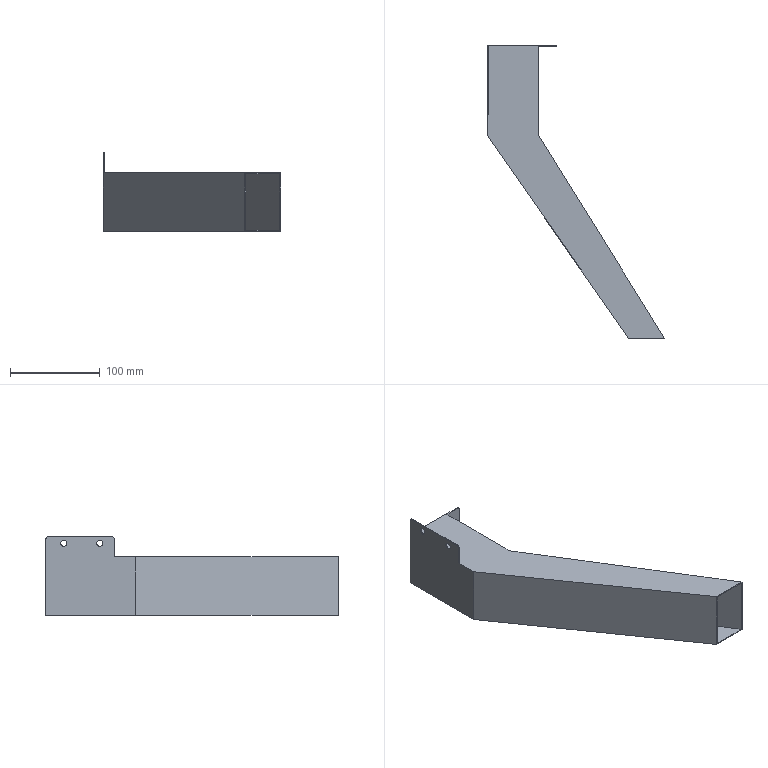Part | NX | 1 solid | 35 faces | box 197 x 325 x 87.5 mm | volume 82670 mm3 | plane 19 | cylinder 12 | cone 4 | commonest cylinder face diameters 6 x4 6.4 x4 7 x4
STEP:
#1=CARTESIAN_POINT('',(1114.,-232.5,-79.28));
#2=VERTEX_POINT('',#1);
#3=CARTESIAN_POINT('',(1271.,-457.5,-79.28));
#4=VERTEX_POINT('',#3);
#5=CARTESIAN_POINT('',(1002.386,-72.544,-79.28));
#6=DIRECTION('',(0.5722,-0.8201,0.));
#7=VECTOR('',#6,1000.);
#8=LINE('',#5,#7);
#9=EDGE_CURVE('',#2,#4,#8,.T.);
#10=ORIENTED_EDGE('',*,*,#9,.F.);
#11=CARTESIAN_POINT('',(1114.,-232.5,-144.28));
#12=VERTEX_POINT('',#11);
#13=CARTESIAN_POINT('',(1114.,-232.5,-79.28));
#14=DIRECTION('',(0.,0.,-1.));
#15=VECTOR('',#14,1000.);
#16=LINE('',#13,#15);
#17=EDGE_CURVE('',#2,#12,#16,.T.);
#18=ORIENTED_EDGE('',*,*,#17,.T.);
#19=CARTESIAN_POINT('',(1271.,-457.5,-144.28));
#20=VERTEX_POINT('',#19);
#21=CARTESIAN_POINT('',(1002.386,-72.544,-144.28));
#22=DIRECTION('',(0.5722,-0.8201,0.));
#23=VECTOR('',#22,1000.);
#24=LINE('',#21,#23);
#25=EDGE_CURVE('',#12,#20,#24,.T.);
#26=ORIENTED_EDGE('',*,*,#25,.T.);
#27=CARTESIAN_POINT('',(1271.,-457.5,-79.28));
#28=DIRECTION('',(0.,0.,1.));
#29=VECTOR('',#28,1000.);
#30=LINE('',#27,#29);
#31=EDGE_CURVE('',#20,#4,#30,.T.);
#32=ORIENTED_EDGE('',*,*,#31,.T.);
#33=EDGE_LOOP('',(#10,#18,#26,#32));
#34=FACE_BOUND('',#33,.T.);
#35=CARTESIAN_POINT('',(1114.,-232.5,-79.28));
#36=DIRECTION('',(-0.8201,-0.5722,0.));
#37=DIRECTION('',(-0.5722,0.8201,0.));
#38=AXIS2_PLACEMENT_3D('',#35,#36,#37);
#39=PLANE('',#38);
#40=ADVANCED_FACE('',(#34),#39,.T.);
#41=CARTESIAN_POINT('',(1114.,-132.5,-144.28));
#42=VERTEX_POINT('',#41);
#43=CARTESIAN_POINT('',(1114.,-132.5,-59.78));
#44=VERTEX_POINT('',#43);
#45=CARTESIAN_POINT('',(1114.,-132.5,-79.28));
#46=DIRECTION('',(0.,0.,1.));
#47=VECTOR('',#46,1000.);
#48=LINE('',#45,#47);
#49=EDGE_CURVE('',#42,#44,#48,.T.);
#50=ORIENTED_EDGE('',*,*,#49,.F.);
#51=CARTESIAN_POINT('',(1114.,-232.5,-144.28));
#52=DIRECTION('',(0.,1.,0.));
#53=VECTOR('',#52,1000.);
#54=LINE('',#51,#53);
#55=EDGE_CURVE('',#12,#42,#54,.T.);
#56=ORIENTED_EDGE('',*,*,#55,.F.);
#57=ORIENTED_EDGE('',*,*,#17,.F.);
#58=CARTESIAN_POINT('',(1114.,-208.721,-79.28));
#59=VERTEX_POINT('',#58);
#60=CARTESIAN_POINT('',(1114.,-232.5,-79.28));
#61=DIRECTION('',(0.,1.,0.));
#62=VECTOR('',#61,1000.);
#63=LINE('',#60,#62);
#64=EDGE_CURVE('',#2,#59,#63,.T.);
#65=ORIENTED_EDGE('',*,*,#64,.T.);
#66=CARTESIAN_POINT('',(1114.,-208.721,-59.78));
#67=VERTEX_POINT('',#66);
#68=CARTESIAN_POINT('',(1114.,-208.721,-79.28));
#69=DIRECTION('',(0.,0.,1.));
#70=VECTOR('',#69,1000.);
#71=LINE('',#68,#70);
#72=EDGE_CURVE('',#59,#67,#71,.T.);
#73=ORIENTED_EDGE('',*,*,#72,.T.);
#74=CARTESIAN_POINT('',(1114.,-205.721,-56.78));
#75=VERTEX_POINT('',#74);
#76=CARTESIAN_POINT('',(1114.,-205.721,-59.78));
#77=DIRECTION('',(-1.,0.,0.));
#78=DIRECTION('',(0.,1.,0.));
#79=AXIS2_PLACEMENT_3D('',#76,#77,#78);
#80=CIRCLE('',#79,3.);
#81=EDGE_CURVE('',#67,#75,#80,.T.);
#82=ORIENTED_EDGE('',*,*,#81,.T.);
#83=CARTESIAN_POINT('',(1114.,-135.5,-56.78));
#84=VERTEX_POINT('',#83);
#85=CARTESIAN_POINT('',(1114.,-72.544,-56.78));
#86=DIRECTION('',(0.,1.,0.));
#87=VECTOR('',#86,1000.);
#88=LINE('',#85,#87);
#89=EDGE_CURVE('',#75,#84,#88,.T.);
#90=ORIENTED_EDGE('',*,*,#89,.T.);
#91=CARTESIAN_POINT('',(1114.,-135.5,-59.78));
#92=DIRECTION('',(1.,0.,0.));
#93=DIRECTION('',(0.,-1.,0.));
#94=AXIS2_PLACEMENT_3D('',#91,#92,#93);
#95=CIRCLE('',#94,3.);
#96=EDGE_CURVE('',#44,#84,#95,.T.);
#97=ORIENTED_EDGE('',*,*,#96,.F.);
#98=EDGE_LOOP('',(#50,#56,#57,#65,#73,#82,#90,#97));
#99=FACE_BOUND('',#98,.T.);
#100=CARTESIAN_POINT('',(1114.,-149.,-64.28));
#101=VERTEX_POINT('',#100);
#102=CARTESIAN_POINT('',(1114.,-156.,-64.28));
#103=VERTEX_POINT('',#102);
#104=CARTESIAN_POINT('',(1114.,-152.5,-64.28));
#105=DIRECTION('',(1.,0.,0.));
#106=DIRECTION('',(0.,-1.,0.));
#107=AXIS2_PLACEMENT_3D('',#104,#105,#106);
#108=CIRCLE('',#107,3.5);
#109=EDGE_CURVE('',#101,#103,#108,.T.);
#110=ORIENTED_EDGE('',*,*,#109,.T.);
#111=CARTESIAN_POINT('',(1114.,-152.5,-64.28));
#112=DIRECTION('',(1.,0.,0.));
#113=DIRECTION('',(0.,-1.,0.));
#114=AXIS2_PLACEMENT_3D('',#111,#112,#113);
#115=CIRCLE('',#114,3.5);
#116=EDGE_CURVE('',#103,#101,#115,.T.);
#117=ORIENTED_EDGE('',*,*,#116,.T.);
#118=EDGE_LOOP('',(#110,#117));
#119=FACE_BOUND('',#118,.T.);
#120=CARTESIAN_POINT('',(1114.,-189.,-64.28));
#121=VERTEX_POINT('',#120);
#122=CARTESIAN_POINT('',(1114.,-196.,-64.28));
#123=VERTEX_POINT('',#122);
#124=CARTESIAN_POINT('',(1114.,-192.5,-64.28));
#125=DIRECTION('',(1.,0.,0.));
#126=DIRECTION('',(0.,-1.,0.));
#127=AXIS2_PLACEMENT_3D('',#124,#125,#126);
#128=CIRCLE('',#127,3.5);
#129=EDGE_CURVE('',#121,#123,#128,.T.);
#130=ORIENTED_EDGE('',*,*,#129,.T.);
#131=CARTESIAN_POINT('',(1114.,-192.5,-64.28));
#132=DIRECTION('',(1.,0.,0.));
#133=DIRECTION('',(0.,-1.,0.));
#134=AXIS2_PLACEMENT_3D('',#131,#132,#133);
#135=CIRCLE('',#134,3.5);
#136=EDGE_CURVE('',#123,#121,#135,.T.);
#137=ORIENTED_EDGE('',*,*,#136,.T.);
#138=EDGE_LOOP('',(#130,#137));
#139=FACE_BOUND('',#138,.T.);
#140=CARTESIAN_POINT('',(1114.,-132.5,-79.28));
#141=DIRECTION('',(-1.,0.,0.));
#142=DIRECTION('',(0.,0.,1.));
#143=AXIS2_PLACEMENT_3D('',#140,#141,#142);
#144=PLANE('',#143);
#145=ADVANCED_FACE('',(#99,#119,#139),#144,.T.);
#146=CARTESIAN_POINT('',(1191.,-132.5,-82.28));
#147=VERTEX_POINT('',#146);
#148=CARTESIAN_POINT('',(1191.,-132.5,-141.28));
#149=VERTEX_POINT('',#148);
#150=CARTESIAN_POINT('',(1191.,-132.5,-130.28));
#151=DIRECTION('',(0.,0.,-1.));
#152=VECTOR('',#151,1000.);
#153=LINE('',#150,#152);
#154=EDGE_CURVE('',#147,#149,#153,.T.);
#155=ORIENTED_EDGE('',*,*,#154,.F.);
#156=CARTESIAN_POINT('',(1191.,-133.5,-82.28));
#157=VERTEX_POINT('',#156);
#158=CARTESIAN_POINT('',(1191.,-132.5,-82.28));
#159=DIRECTION('',(0.,-1.,0.));
#160=VECTOR('',#159,1000.);
#161=LINE('',#158,#160);
#162=EDGE_CURVE('',#147,#157,#161,.T.);
#163=ORIENTED_EDGE('',*,*,#162,.T.);
#164=CARTESIAN_POINT('',(1191.,-133.5,-141.28));
#165=VERTEX_POINT('',#164);
#166=CARTESIAN_POINT('',(1191.,-133.5,-130.28));
#167=DIRECTION('',(0.,0.,-1.));
#168=VECTOR('',#167,1000.);
#169=LINE('',#166,#168);
#170=EDGE_CURVE('',#157,#165,#169,.T.);
#171=ORIENTED_EDGE('',*,*,#170,.T.);
#172=CARTESIAN_POINT('',(1191.,-132.5,-141.28));
#173=DIRECTION('',(0.,-1.,0.));
#174=VECTOR('',#173,1000.);
#175=LINE('',#172,#174);
#176=EDGE_CURVE('',#149,#165,#175,.T.);
#177=ORIENTED_EDGE('',*,*,#176,.F.);
#178=EDGE_LOOP('',(#155,#163,#171,#177));
#179=FACE_BOUND('',#178,.T.);
#180=CARTESIAN_POINT('',(1191.,-132.5,-82.28));
#181=DIRECTION('',(1.,0.,0.));
#182=DIRECTION('',(0.,1.,0.));
#183=AXIS2_PLACEMENT_3D('',#180,#181,#182);
#184=PLANE('',#183);
#185=ADVANCED_FACE('',(#179),#184,.T.);
#186=CARTESIAN_POINT('',(1171.,-133.5,-79.28));
#187=VERTEX_POINT('',#186);
#188=CARTESIAN_POINT('',(1171.,-232.5,-79.28));
#189=VERTEX_POINT('',#188);
#190=CARTESIAN_POINT('',(1171.,-132.5,-79.28));
#191=DIRECTION('',(0.,-1.,0.));
#192=VECTOR('',#191,1000.);
#193=LINE('',#190,#192);
#194=EDGE_CURVE('',#187,#189,#193,.T.);
#195=ORIENTED_EDGE('',*,*,#194,.T.);
#196=CARTESIAN_POINT('',(1171.,-232.5,-144.28));
#197=VERTEX_POINT('',#196);
#198=CARTESIAN_POINT('',(1171.,-232.5,-79.28));
#199=DIRECTION('',(0.,0.,-1.));
#200=VECTOR('',#199,1000.);
#201=LINE('',#198,#200);
#202=EDGE_CURVE('',#189,#197,#201,.T.);
#203=ORIENTED_EDGE('',*,*,#202,.T.);
#204=CARTESIAN_POINT('',(1171.,-133.5,-144.28));
#205=VERTEX_POINT('',#204);
#206=CARTESIAN_POINT('',(1171.,-132.5,-144.28));
#207=DIRECTION('',(0.,-1.,0.));
#208=VECTOR('',#207,1000.);
#209=LINE('',#206,#208);
#210=EDGE_CURVE('',#205,#197,#209,.T.);
#211=ORIENTED_EDGE('',*,*,#210,.F.);
#212=CARTESIAN_POINT('',(1171.,-133.5,-79.28));
#213=DIRECTION('',(0.,0.,1.));
#214=VECTOR('',#213,1000.);
#215=LINE('',#212,#214);
#216=EDGE_CURVE('',#205,#187,#215,.T.);
#217=ORIENTED_EDGE('',*,*,#216,.T.);
#218=EDGE_LOOP('',(#195,#203,#211,#217));
#219=FACE_BOUND('',#218,.T.);
#220=CARTESIAN_POINT('',(1171.,-232.5,-79.28));
#221=DIRECTION('',(1.,0.,0.));
#222=DIRECTION('',(0.,1.,0.));
#223=AXIS2_PLACEMENT_3D('',#220,#221,#222);
#224=PLANE('',#223);
#225=ADVANCED_FACE('',(#219),#224,.T.);
#226=CARTESIAN_POINT('',(1311.,-457.5,-79.28));
#227=VERTEX_POINT('',#226);
#228=CARTESIAN_POINT('',(1071.472,-72.544,-79.28));
#229=DIRECTION('',(0.5283,-0.8491,0.));
#230=VECTOR('',#229,1000.);
#231=LINE('',#228,#230);
#232=EDGE_CURVE('',#189,#227,#231,.T.);
#233=ORIENTED_EDGE('',*,*,#232,.T.);
#234=CARTESIAN_POINT('',(1311.,-457.5,-144.28));
#235=VERTEX_POINT('',#234);
#236=CARTESIAN_POINT('',(1311.,-457.5,-79.28));
#237=DIRECTION('',(0.,0.,-1.));
#238=VECTOR('',#237,1000.);
#239=LINE('',#236,#238);
#240=EDGE_CURVE('',#227,#235,#239,.T.);
#241=ORIENTED_EDGE('',*,*,#240,.T.);
#242=CARTESIAN_POINT('',(1071.472,-72.544,-144.28));
#243=DIRECTION('',(0.5283,-0.8491,0.));
#244=VECTOR('',#243,1000.);
#245=LINE('',#242,#244);
#246=EDGE_CURVE('',#197,#235,#245,.T.);
#247=ORIENTED_EDGE('',*,*,#246,.F.);
#248=ORIENTED_EDGE('',*,*,#202,.F.);
#249=EDGE_LOOP('',(#233,#241,#247,#248));
#250=FACE_BOUND('',#249,.T.);
#251=CARTESIAN_POINT('',(1311.,-457.5,-79.28));
#252=DIRECTION('',(0.8491,0.5283,0.));
#253=DIRECTION('',(0.,0.,-1.));
#254=AXIS2_PLACEMENT_3D('',#251,#252,#253);
#255=PLANE('',#254);
#256=ADVANCED_FACE('',(#250),#255,.T.);
#257=CARTESIAN_POINT('',(1140.033,-457.5,-79.28));
#258=DIRECTION('',(1.,0.,0.));
#259=VECTOR('',#258,1000.);
#260=LINE('',#257,#259);
#261=EDGE_CURVE('',#4,#227,#260,.T.);
#262=ORIENTED_EDGE('',*,*,#261,.F.);
#263=ORIENTED_EDGE('',*,*,#31,.F.);
#264=CARTESIAN_POINT('',(1140.033,-457.5,-144.28));
#265=DIRECTION('',(1.,0.,0.));
#266=VECTOR('',#265,1000.);
#267=LINE('',#264,#266);
#268=EDGE_CURVE('',#20,#235,#267,.T.);
#269=ORIENTED_EDGE('',*,*,#268,.T.);
#270=ORIENTED_EDGE('',*,*,#240,.F.);
#271=EDGE_LOOP('',(#262,#263,#269,#270));
#272=FACE_BOUND('',#271,.T.);
#273=CARTESIAN_POINT('',(1309.822,-457.5,-80.28));
#274=VERTEX_POINT('',#273);
#275=CARTESIAN_POINT('',(1309.822,-457.5,-143.28));
#276=VERTEX_POINT('',#275);
#277=CARTESIAN_POINT('',(1309.822,-457.5,-79.28));
#278=DIRECTION('',(0.,0.,-1.));
#279=VECTOR('',#278,1000.);
#280=LINE('',#277,#279);
#281=EDGE_CURVE('',#274,#276,#280,.T.);
#282=ORIENTED_EDGE('',*,*,#281,.T.);
#283=CARTESIAN_POINT('',(1272.219,-457.5,-143.28));
#284=VERTEX_POINT('',#283);
#285=CARTESIAN_POINT('',(1140.033,-457.5,-143.28));
#286=DIRECTION('',(1.,0.,0.));
#287=VECTOR('',#286,1000.);
#288=LINE('',#285,#287);
#289=EDGE_CURVE('',#284,#276,#288,.T.);
#290=ORIENTED_EDGE('',*,*,#289,.F.);
#291=CARTESIAN_POINT('',(1272.219,-457.5,-80.28));
#292=VERTEX_POINT('',#291);
#293=CARTESIAN_POINT('',(1272.219,-457.5,-79.28));
#294=DIRECTION('',(0.,0.,1.));
#295=VECTOR('',#294,1000.);
#296=LINE('',#293,#295);
#297=EDGE_CURVE('',#284,#292,#296,.T.);
#298=ORIENTED_EDGE('',*,*,#297,.T.);
#299=CARTESIAN_POINT('',(1140.033,-457.5,-80.28));
#300=DIRECTION('',(1.,0.,0.));
#301=VECTOR('',#300,1000.);
#302=LINE('',#299,#301);
#303=EDGE_CURVE('',#292,#274,#302,.T.);
#304=ORIENTED_EDGE('',*,*,#303,.T.);
#305=EDGE_LOOP('',(#282,#290,#298,#304));
#306=FACE_BOUND('',#305,.T.);
#307=CARTESIAN_POINT('',(1271.,-457.5,-79.28));
#308=DIRECTION('',(0.,-1.,0.));
#309=DIRECTION('',(0.,0.,-1.));
#310=AXIS2_PLACEMENT_3D('',#307,#308,#309);
#311=PLANE('',#310);
#312=ADVANCED_FACE('',(#272,#306),#311,.T.);
#313=ORIENTED_EDGE('',*,*,#303,.F.);
#314=CARTESIAN_POINT('',(1115.,-232.186,-80.28));
#315=VERTEX_POINT('',#314);
#316=CARTESIAN_POINT('',(1003.606,-72.544,-80.28));
#317=DIRECTION('',(-0.5722,0.8201,0.));
#318=VECTOR('',#317,1000.);
#319=LINE('',#316,#318);
#320=EDGE_CURVE('',#292,#315,#319,.T.);
#321=ORIENTED_EDGE('',*,*,#320,.T.);
#322=CARTESIAN_POINT('',(1115.,-132.5,-80.28));
#323=VERTEX_POINT('',#322);
#324=CARTESIAN_POINT('',(1115.,-72.544,-80.28));
#325=DIRECTION('',(0.,1.,0.));
#326=VECTOR('',#325,1000.);
#327=LINE('',#324,#326);
#328=EDGE_CURVE('',#315,#323,#327,.T.);
#329=ORIENTED_EDGE('',*,*,#328,.T.);
#330=CARTESIAN_POINT('',(1170.,-132.5,-80.28));
#331=VERTEX_POINT('',#330);
#332=CARTESIAN_POINT('',(1140.033,-132.5,-80.28));
#333=DIRECTION('',(1.,0.,0.));
#334=VECTOR('',#333,1000.);
#335=LINE('',#332,#334);
#336=EDGE_CURVE('',#323,#331,#335,.T.);
#337=ORIENTED_EDGE('',*,*,#336,.T.);
#338=CARTESIAN_POINT('',(1170.,-232.786,-80.28));
#339=VERTEX_POINT('',#338);
#340=CARTESIAN_POINT('',(1170.,-132.5,-80.28));
#341=DIRECTION('',(0.,-1.,0.));
#342=VECTOR('',#341,1000.);
#343=LINE('',#340,#342);
#344=EDGE_CURVE('',#331,#339,#343,.T.);
#345=ORIENTED_EDGE('',*,*,#344,.T.);
#346=CARTESIAN_POINT('',(1070.294,-72.544,-80.28));
#347=DIRECTION('',(0.5283,-0.8491,0.));
#348=VECTOR('',#347,1000.);
#349=LINE('',#346,#348);
#350=EDGE_CURVE('',#339,#274,#349,.T.);
#351=ORIENTED_EDGE('',*,*,#350,.T.);
#352=EDGE_LOOP('',(#313,#321,#329,#337,#345,#351));
#353=FACE_BOUND('',#352,.T.);
#354=CARTESIAN_POINT('',(1140.033,-72.544,-80.28));
#355=DIRECTION('',(0.,0.,1.));
#356=DIRECTION('',(1.,0.,0.));
#357=AXIS2_PLACEMENT_3D('',#354,#355,#356);
#358=PLANE('',#357);
#359=ADVANCED_FACE('',(#353),#358,.F.);
#360=CARTESIAN_POINT('',(1170.,-232.786,-143.28));
#361=VERTEX_POINT('',#360);
#362=CARTESIAN_POINT('',(1070.294,-72.544,-143.28));
#363=DIRECTION('',(0.5283,-0.8491,0.));
#364=VECTOR('',#363,1000.);
#365=LINE('',#362,#364);
#366=EDGE_CURVE('',#361,#276,#365,.T.);
#367=ORIENTED_EDGE('',*,*,#366,.F.);
#368=CARTESIAN_POINT('',(1170.,-132.5,-143.28));
#369=VERTEX_POINT('',#368);
#370=CARTESIAN_POINT('',(1170.,-72.544,-143.28));
#371=DIRECTION('',(0.,-1.,0.));
#372=VECTOR('',#371,1000.);
#373=LINE('',#370,#372);
#374=EDGE_CURVE('',#369,#361,#373,.T.);
#375=ORIENTED_EDGE('',*,*,#374,.F.);
#376=CARTESIAN_POINT('',(1115.,-132.5,-143.28));
#377=VERTEX_POINT('',#376);
#378=CARTESIAN_POINT('',(1140.033,-132.5,-143.28));
#379=DIRECTION('',(-1.,0.,0.));
#380=VECTOR('',#379,1000.);
#381=LINE('',#378,#380);
#382=EDGE_CURVE('',#369,#377,#381,.T.);
#383=ORIENTED_EDGE('',*,*,#382,.T.);
#384=CARTESIAN_POINT('',(1115.,-232.186,-143.28));
#385=VERTEX_POINT('',#384);
#386=CARTESIAN_POINT('',(1115.,-72.544,-143.28));
#387=DIRECTION('',(0.,1.,0.));
#388=VECTOR('',#387,1000.);
#389=LINE('',#386,#388);
#390=EDGE_CURVE('',#385,#377,#389,.T.);
#391=ORIENTED_EDGE('',*,*,#390,.F.);
#392=CARTESIAN_POINT('',(1003.606,-72.544,-143.28));
#393=DIRECTION('',(-0.5722,0.8201,0.));
#394=VECTOR('',#393,1000.);
#395=LINE('',#392,#394);
#396=EDGE_CURVE('',#284,#385,#395,.T.);
#397=ORIENTED_EDGE('',*,*,#396,.F.);
#398=ORIENTED_EDGE('',*,*,#289,.T.);
#399=EDGE_LOOP('',(#367,#375,#383,#391,#397,#398));
#400=FACE_BOUND('',#399,.T.);
#401=CARTESIAN_POINT('',(1140.033,-72.544,-143.28));
#402=DIRECTION('',(0.,0.,1.));
#403=DIRECTION('',(1.,0.,0.));
#404=AXIS2_PLACEMENT_3D('',#401,#402,#403);
#405=PLANE('',#404);
#406=ADVANCED_FACE('',(#400),#405,.T.);
#407=ORIENTED_EDGE('',*,*,#297,.F.);
#408=ORIENTED_EDGE('',*,*,#396,.T.);
#409=CARTESIAN_POINT('',(1115.,-232.186,-79.28));
#410=DIRECTION('',(0.,0.,1.));
#411=VECTOR('',#410,1000.);
#412=LINE('',#409,#411);
#413=EDGE_CURVE('',#385,#315,#412,.T.);
#414=ORIENTED_EDGE('',*,*,#413,.T.);
#415=ORIENTED_EDGE('',*,*,#320,.F.);
#416=EDGE_LOOP('',(#407,#408,#414,#415));
#417=FACE_BOUND('',#416,.T.);
#418=CARTESIAN_POINT('',(1114.82,-231.928,-79.28));
#419=DIRECTION('',(-0.8201,-0.5722,0.));
#420=DIRECTION('',(-0.5722,0.8201,0.));
#421=AXIS2_PLACEMENT_3D('',#418,#419,#420);
#422=PLANE('',#421);
#423=ADVANCED_FACE('',(#417),#422,.F.);
#424=ORIENTED_EDGE('',*,*,#413,.F.);
#425=ORIENTED_EDGE('',*,*,#390,.T.);
#426=CARTESIAN_POINT('',(1115.,-132.5,-79.28));
#427=DIRECTION('',(0.,0.,1.));
#428=VECTOR('',#427,1000.);
#429=LINE('',#426,#428);
#430=EDGE_CURVE('',#377,#323,#429,.T.);
#431=ORIENTED_EDGE('',*,*,#430,.T.);
#432=ORIENTED_EDGE('',*,*,#328,.F.);
#433=EDGE_LOOP('',(#424,#425,#431,#432));
#434=FACE_BOUND('',#433,.T.);
#435=CARTESIAN_POINT('',(1115.,-132.5,-79.28));
#436=DIRECTION('',(-1.,0.,0.));
#437=DIRECTION('',(0.,0.,1.));
#438=AXIS2_PLACEMENT_3D('',#435,#436,#437);
#439=PLANE('',#438);
#440=ADVANCED_FACE('',(#434),#439,.F.);
#441=CARTESIAN_POINT('',(1188.,-132.5,-144.28));
#442=VERTEX_POINT('',#441);
#443=CARTESIAN_POINT('',(1188.,-132.5,-141.28));
#444=DIRECTION('',(0.,1.,0.));
#445=DIRECTION('',(1.,0.,0.));
#446=AXIS2_PLACEMENT_3D('',#443,#444,#445);
#447=CIRCLE('',#446,3.);
#448=EDGE_CURVE('',#149,#442,#447,.T.);
#449=ORIENTED_EDGE('',*,*,#448,.F.);
#450=ORIENTED_EDGE('',*,*,#176,.T.);
#451=CARTESIAN_POINT('',(1188.,-133.5,-144.28));
#452=VERTEX_POINT('',#451);
#453=CARTESIAN_POINT('',(1188.,-133.5,-141.28));
#454=DIRECTION('',(0.,1.,0.));
#455=DIRECTION('',(1.,0.,0.));
#456=AXIS2_PLACEMENT_3D('',#453,#454,#455);
#457=CIRCLE('',#456,3.);
#458=EDGE_CURVE('',#165,#452,#457,.T.);
#459=ORIENTED_EDGE('',*,*,#458,.T.);
#460=CARTESIAN_POINT('',(1188.,-132.5,-144.28));
#461=DIRECTION('',(0.,-1.,0.));
#462=VECTOR('',#461,1000.);
#463=LINE('',#460,#462);
#464=EDGE_CURVE('',#442,#452,#463,.T.);
#465=ORIENTED_EDGE('',*,*,#464,.F.);
#466=EDGE_LOOP('',(#449,#450,#459,#465));
#467=FACE_BOUND('',#466,.T.);
#468=CARTESIAN_POINT('',(1188.,-132.5,-141.28));
#469=DIRECTION('',(0.,1.,0.));
#470=DIRECTION('',(1.,0.,0.));
#471=AXIS2_PLACEMENT_3D('',#468,#469,#470);
#472=CYLINDRICAL_SURFACE('',#471,3.);
#473=ADVANCED_FACE('',(#467),#472,.T.);
#474=ORIENTED_EDGE('',*,*,#374,.T.);
#475=CARTESIAN_POINT('',(1170.,-232.786,-79.28));
#476=DIRECTION('',(0.,0.,-1.));
#477=VECTOR('',#476,1000.);
#478=LINE('',#475,#477);
#479=EDGE_CURVE('',#339,#361,#478,.T.);
#480=ORIENTED_EDGE('',*,*,#479,.F.);
#481=ORIENTED_EDGE('',*,*,#344,.F.);
#482=CARTESIAN_POINT('',(1170.,-132.5,-79.28));
#483=DIRECTION('',(0.,0.,-1.));
#484=VECTOR('',#483,1000.);
#485=LINE('',#482,#484);
#486=EDGE_CURVE('',#331,#369,#485,.T.);
#487=ORIENTED_EDGE('',*,*,#486,.T.);
#488=EDGE_LOOP('',(#474,#480,#481,#487));
#489=FACE_BOUND('',#488,.T.);
#490=CARTESIAN_POINT('',(1170.,-232.5,-79.28));
#491=DIRECTION('',(1.,0.,0.));
#492=DIRECTION('',(0.,1.,0.));
#493=AXIS2_PLACEMENT_3D('',#490,#491,#492);
#494=PLANE('',#493);
#495=ADVANCED_FACE('',(#489),#494,.F.);
#496=ORIENTED_EDGE('',*,*,#479,.T.);
#497=ORIENTED_EDGE('',*,*,#366,.T.);
#498=ORIENTED_EDGE('',*,*,#281,.F.);
#499=ORIENTED_EDGE('',*,*,#350,.F.);
#500=EDGE_LOOP('',(#496,#497,#498,#499));
#501=FACE_BOUND('',#500,.T.);
#502=CARTESIAN_POINT('',(1310.151,-458.028,-79.28));
#503=DIRECTION('',(0.8491,0.5283,0.));
#504=DIRECTION('',(0.,0.,-1.));
#505=AXIS2_PLACEMENT_3D('',#502,#503,#504);
#506=PLANE('',#505);
#507=ADVANCED_FACE('',(#501),#506,.F.);
#508=CARTESIAN_POINT('',(1120.,-132.5,-144.28));
#509=DIRECTION('',(1.,0.,0.));
#510=VECTOR('',#509,1000.);
#511=LINE('',#508,#510);
#512=EDGE_CURVE('',#42,#442,#511,.T.);
#513=ORIENTED_EDGE('',*,*,#512,.F.);
#514=ORIENTED_EDGE('',*,*,#49,.T.);
#515=CARTESIAN_POINT('',(1115.,-132.5,-59.78));
#516=VERTEX_POINT('',#515);
#517=CARTESIAN_POINT('',(1140.033,-132.5,-59.78));
#518=DIRECTION('',(1.,0.,0.));
#519=VECTOR('',#518,1000.);
#520=LINE('',#517,#519);
#521=EDGE_CURVE('',#44,#516,#520,.T.);
#522=ORIENTED_EDGE('',*,*,#521,.T.);
#523=CARTESIAN_POINT('',(1115.,-132.5,-79.28));
#524=VERTEX_POINT('',#523);
#525=CARTESIAN_POINT('',(1115.,-132.5,-79.28));
#526=DIRECTION('',(0.,0.,1.));
#527=VECTOR('',#526,1000.);
#528=LINE('',#525,#527);
#529=EDGE_CURVE('',#524,#516,#528,.T.);
#530=ORIENTED_EDGE('',*,*,#529,.F.);
#531=CARTESIAN_POINT('',(1188.,-132.5,-79.28));
#532=VERTEX_POINT('',#531);
#533=CARTESIAN_POINT('',(1114.,-132.5,-79.28));
#534=DIRECTION('',(1.,0.,0.));
#535=VECTOR('',#534,1000.);
#536=LINE('',#533,#535);
#537=EDGE_CURVE('',#524,#532,#536,.T.);
#538=ORIENTED_EDGE('',*,*,#537,.T.);
#539=CARTESIAN_POINT('',(1188.,-132.5,-82.28));
#540=DIRECTION('',(0.,1.,0.));
#541=DIRECTION('',(1.,0.,0.));
#542=AXIS2_PLACEMENT_3D('',#539,#540,#541);
#543=CIRCLE('',#542,3.);
#544=EDGE_CURVE('',#532,#147,#543,.T.);
#545=ORIENTED_EDGE('',*,*,#544,.T.);
#546=ORIENTED_EDGE('',*,*,#154,.T.);
#547=ORIENTED_EDGE('',*,*,#448,.T.);
#548=EDGE_LOOP('',(#513,#514,#522,#530,#538,#545,#546,#547));
#549=FACE_BOUND('',#548,.T.);
#550=ORIENTED_EDGE('',*,*,#382,.F.);
#551=ORIENTED_EDGE('',*,*,#486,.F.);
#552=ORIENTED_EDGE('',*,*,#336,.F.);
#553=ORIENTED_EDGE('',*,*,#430,.F.);
#554=EDGE_LOOP('',(#550,#551,#552,#553));
#555=FACE_BOUND('',#554,.T.);
#556=CARTESIAN_POINT('',(1183.7,-132.5,-96.03));
#557=VERTEX_POINT('',#556);
#558=CARTESIAN_POINT('',(1177.3,-132.5,-96.03));
#559=VERTEX_POINT('',#558);
#560=CARTESIAN_POINT('',(1180.5,-132.5,-96.03));
#561=DIRECTION('',(0.,-1.,0.));
#562=DIRECTION('',(-1.,0.,0.));
#563=AXIS2_PLACEMENT_3D('',#560,#561,#562);
#564=CIRCLE('',#563,3.2);
#565=EDGE_CURVE('',#557,#559,#564,.T.);
#566=ORIENTED_EDGE('',*,*,#565,.T.);
#567=CARTESIAN_POINT('',(1180.5,-132.5,-96.03));
#568=DIRECTION('',(0.,-1.,0.));
#569=DIRECTION('',(-1.,0.,0.));
#570=AXIS2_PLACEMENT_3D('',#567,#568,#569);
#571=CIRCLE('',#570,3.2);
#572=EDGE_CURVE('',#559,#557,#571,.T.);
#573=ORIENTED_EDGE('',*,*,#572,.T.);
#574=EDGE_LOOP('',(#566,#573));
#575=FACE_BOUND('',#574,.T.);
#576=CARTESIAN_POINT('',(1183.7,-132.5,-127.53));
#577=VERTEX_POINT('',#576);
#578=CARTESIAN_POINT('',(1177.3,-132.5,-127.53));
#579=VERTEX_POINT('',#578);
#580=CARTESIAN_POINT('',(1180.5,-132.5,-127.53));
#581=DIRECTION('',(0.,-1.,0.));
#582=DIRECTION('',(-1.,0.,0.));
#583=AXIS2_PLACEMENT_3D('',#580,#581,#582);
#584=CIRCLE('',#583,3.2);
#585=EDGE_CURVE('',#577,#579,#584,.T.);
#586=ORIENTED_EDGE('',*,*,#585,.T.);
#587=CARTESIAN_POINT('',(1180.5,-132.5,-127.53));
#588=DIRECTION('',(0.,-1.,0.));
#589=DIRECTION('',(-1.,0.,0.));
#590=AXIS2_PLACEMENT_3D('',#587,#588,#589);
#591=CIRCLE('',#590,3.2);
#592=EDGE_CURVE('',#579,#577,#591,.T.);
#593=ORIENTED_EDGE('',*,*,#592,.T.);
#594=EDGE_LOOP('',(#586,#593));
#595=FACE_BOUND('',#594,.T.);
#596=CARTESIAN_POINT('',(1171.,-132.5,-79.28));
#597=DIRECTION('',(0.,1.,0.));
#598=DIRECTION('',(1.,0.,0.));
#599=AXIS2_PLACEMENT_3D('',#596,#597,#598);
#600=PLANE('',#599);
#601=ADVANCED_FACE('',(#549,#555,#575,#595),#600,.T.);
#602=ORIENTED_EDGE('',*,*,#544,.F.);
#603=CARTESIAN_POINT('',(1188.,-133.5,-79.28));
#604=VERTEX_POINT('',#603);
#605=CARTESIAN_POINT('',(1188.,-132.5,-79.28));
#606=DIRECTION('',(0.,-1.,0.));
#607=VECTOR('',#606,1000.);
#608=LINE('',#605,#607);
#609=EDGE_CURVE('',#532,#604,#608,.T.);
#610=ORIENTED_EDGE('',*,*,#609,.T.);
#611=CARTESIAN_POINT('',(1188.,-133.5,-82.28));
#612=DIRECTION('',(0.,1.,0.));
#613=DIRECTION('',(1.,0.,0.));
#614=AXIS2_PLACEMENT_3D('',#611,#612,#613);
#615=CIRCLE('',#614,3.);
#616=EDGE_CURVE('',#604,#157,#615,.T.);
#617=ORIENTED_EDGE('',*,*,#616,.T.);
#618=ORIENTED_EDGE('',*,*,#162,.F.);
#619=EDGE_LOOP('',(#602,#610,#617,#618));
#620=FACE_BOUND('',#619,.T.);
#621=CARTESIAN_POINT('',(1188.,-132.5,-82.28));
#622=DIRECTION('',(0.,1.,0.));
#623=DIRECTION('',(1.,0.,0.));
#624=AXIS2_PLACEMENT_3D('',#621,#622,#623);
#625=CYLINDRICAL_SURFACE('',#624,3.);
#626=ADVANCED_FACE('',(#620),#625,.T.);
#627=CARTESIAN_POINT('',(1183.7,-133.5,-96.03));
#628=VERTEX_POINT('',#627);
#629=CARTESIAN_POINT('',(1177.3,-133.5,-96.03));
#630=VERTEX_POINT('',#629);
#631=CARTESIAN_POINT('',(1180.5,-133.5,-96.03));
#632=DIRECTION('',(0.,-1.,0.));
#633=DIRECTION('',(-1.,0.,0.));
#634=AXIS2_PLACEMENT_3D('',#631,#632,#633);
#635=CIRCLE('',#634,3.2);
#636=EDGE_CURVE('',#628,#630,#635,.T.);
#637=ORIENTED_EDGE('',*,*,#636,.T.);
#638=CARTESIAN_POINT('',(1177.3,-132.5,-96.03));
#639=DIRECTION('',(0.,-1.,0.));
#640=VECTOR('',#639,1000.);
#641=LINE('',#638,#640);
#642=EDGE_CURVE('',#630,#559,#641,.F.);
#643=ORIENTED_EDGE('',*,*,#642,.T.);
#644=ORIENTED_EDGE('',*,*,#565,.F.);
#645=CARTESIAN_POINT('',(1183.7,-132.5,-96.03));
#646=DIRECTION('',(0.,-1.,0.));
#647=VECTOR('',#646,1000.);
#648=LINE('',#645,#647);
#649=EDGE_CURVE('',#628,#557,#648,.F.);
#650=ORIENTED_EDGE('',*,*,#649,.F.);
#651=EDGE_LOOP('',(#637,#643,#644,#650));
#652=FACE_BOUND('',#651,.T.);
#653=CARTESIAN_POINT('',(1180.5,-132.5,-96.03));
#654=DIRECTION('',(0.,-1.,0.));
#655=DIRECTION('',(-1.,0.,0.));
#656=AXIS2_PLACEMENT_3D('',#653,#654,#655);
#657=CYLINDRICAL_SURFACE('',#656,3.2);
#658=ADVANCED_FACE('',(#652),#657,.F.);
#659=ORIENTED_EDGE('',*,*,#170,.F.);
#660=ORIENTED_EDGE('',*,*,#616,.F.);
#661=CARTESIAN_POINT('',(1120.,-133.5,-79.28));
#662=DIRECTION('',(1.,0.,0.));
#663=VECTOR('',#662,1000.);
#664=LINE('',#661,#663);
#665=EDGE_CURVE('',#187,#604,#664,.T.);
#666=ORIENTED_EDGE('',*,*,#665,.F.);
#667=ORIENTED_EDGE('',*,*,#216,.F.);
#668=CARTESIAN_POINT('',(1120.,-133.5,-144.28));
#669=DIRECTION('',(1.,0.,0.));
#670=VECTOR('',#669,1000.);
#671=LINE('',#668,#670);
#672=EDGE_CURVE('',#205,#452,#671,.T.);
#673=ORIENTED_EDGE('',*,*,#672,.T.);
#674=ORIENTED_EDGE('',*,*,#458,.F.);
#675=EDGE_LOOP('',(#659,#660,#666,#667,#673,#674));
#676=FACE_BOUND('',#675,.T.);
#677=ORIENTED_EDGE('',*,*,#636,.F.);
#678=CARTESIAN_POINT('',(1180.5,-133.5,-96.03));
#679=DIRECTION('',(0.,-1.,0.));
#680=DIRECTION('',(-1.,0.,0.));
#681=AXIS2_PLACEMENT_3D('',#678,#679,#680);
#682=CIRCLE('',#681,3.2);
#683=EDGE_CURVE('',#630,#628,#682,.T.);
#684=ORIENTED_EDGE('',*,*,#683,.F.);
#685=EDGE_LOOP('',(#677,#684));
#686=FACE_BOUND('',#685,.T.);
#687=CARTESIAN_POINT('',(1183.7,-133.5,-127.53));
#688=VERTEX_POINT('',#687);
#689=CARTESIAN_POINT('',(1177.3,-133.5,-127.53));
#690=VERTEX_POINT('',#689);
#691=CARTESIAN_POINT('',(1180.5,-133.5,-127.53));
#692=DIRECTION('',(0.,-1.,0.));
#693=DIRECTION('',(-1.,0.,0.));
#694=AXIS2_PLACEMENT_3D('',#691,#692,#693);
#695=CIRCLE('',#694,3.2);
#696=EDGE_CURVE('',#688,#690,#695,.T.);
#697=ORIENTED_EDGE('',*,*,#696,.F.);
#698=CARTESIAN_POINT('',(1180.5,-133.5,-127.53));
#699=DIRECTION('',(0.,-1.,0.));
#700=DIRECTION('',(-1.,0.,0.));
#701=AXIS2_PLACEMENT_3D('',#698,#699,#700);
#702=CIRCLE('',#701,3.2);
#703=EDGE_CURVE('',#690,#688,#702,.T.);
#704=ORIENTED_EDGE('',*,*,#703,.F.);
#705=EDGE_LOOP('',(#697,#704));
#706=FACE_BOUND('',#705,.T.);
#707=CARTESIAN_POINT('',(1138.223,-133.5,-115.593));
#708=DIRECTION('',(0.,1.,0.));
#709=DIRECTION('',(1.,0.,0.));
#710=AXIS2_PLACEMENT_3D('',#707,#708,#709);
#711=PLANE('',#710);
#712=ADVANCED_FACE('',(#676,#686,#706),#711,.F.);
#713=ORIENTED_EDGE('',*,*,#696,.T.);
#714=CARTESIAN_POINT('',(1177.3,-132.5,-127.53));
#715=DIRECTION('',(0.,-1.,0.));
#716=VECTOR('',#715,1000.);
#717=LINE('',#714,#716);
#718=EDGE_CURVE('',#690,#579,#717,.F.);
#719=ORIENTED_EDGE('',*,*,#718,.T.);
#720=ORIENTED_EDGE('',*,*,#585,.F.);
#721=CARTESIAN_POINT('',(1183.7,-132.5,-127.53));
#722=DIRECTION('',(0.,-1.,0.));
#723=VECTOR('',#722,1000.);
#724=LINE('',#721,#723);
#725=EDGE_CURVE('',#688,#577,#724,.F.);
#726=ORIENTED_EDGE('',*,*,#725,.F.);
#727=EDGE_LOOP('',(#713,#719,#720,#726));
#728=FACE_BOUND('',#727,.T.);
#729=CARTESIAN_POINT('',(1180.5,-132.5,-127.53));
#730=DIRECTION('',(0.,-1.,0.));
#731=DIRECTION('',(-1.,0.,0.));
#732=AXIS2_PLACEMENT_3D('',#729,#730,#731);
#733=CYLINDRICAL_SURFACE('',#732,3.2);
#734=ADVANCED_FACE('',(#728),#733,.F.);
#735=CARTESIAN_POINT('',(1114.8,-149.,-64.28));
#736=VERTEX_POINT('',#735);
#737=CARTESIAN_POINT('',(1114.8,-156.,-64.28));
#738=VERTEX_POINT('',#737);
#739=CARTESIAN_POINT('',(1114.8,-152.5,-64.28));
#740=DIRECTION('',(1.,0.,0.));
#741=DIRECTION('',(0.,-1.,0.));
#742=AXIS2_PLACEMENT_3D('',#739,#740,#741);
#743=CIRCLE('',#742,3.5);
#744=EDGE_CURVE('',#736,#738,#743,.T.);
#745=ORIENTED_EDGE('',*,*,#744,.T.);
#746=CARTESIAN_POINT('',(1115.,-156.,-64.28));
#747=DIRECTION('',(1.,0.,0.));
#748=VECTOR('',#747,1000.);
#749=LINE('',#746,#748);
#750=EDGE_CURVE('',#738,#103,#749,.F.);
#751=ORIENTED_EDGE('',*,*,#750,.T.);
#752=ORIENTED_EDGE('',*,*,#109,.F.);
#753=CARTESIAN_POINT('',(1115.,-149.,-64.28));
#754=DIRECTION('',(1.,0.,0.));
#755=VECTOR('',#754,1000.);
#756=LINE('',#753,#755);
#757=EDGE_CURVE('',#736,#101,#756,.F.);
#758=ORIENTED_EDGE('',*,*,#757,.F.);
#759=EDGE_LOOP('',(#745,#751,#752,#758));
#760=FACE_BOUND('',#759,.T.);
#761=CARTESIAN_POINT('',(1115.,-152.5,-64.28));
#762=DIRECTION('',(1.,0.,0.));
#763=DIRECTION('',(0.,-1.,0.));
#764=AXIS2_PLACEMENT_3D('',#761,#762,#763);
#765=CYLINDRICAL_SURFACE('',#764,3.5);
#766=ADVANCED_FACE('',(#760),#765,.F.);
#767=ORIENTED_EDGE('',*,*,#744,.F.);
#768=CARTESIAN_POINT('',(1115.,-148.8,-64.28));
#769=VERTEX_POINT('',#768);
#770=CARTESIAN_POINT('',(1114.8,-149.,-64.28));
#771=DIRECTION('',(0.7071,0.7071,0.));
#772=VECTOR('',#771,1000.);
#773=LINE('',#770,#772);
#774=EDGE_CURVE('',#769,#736,#773,.F.);
#775=ORIENTED_EDGE('',*,*,#774,.F.);
#776=CARTESIAN_POINT('',(1115.,-156.2,-64.28));
#777=VERTEX_POINT('',#776);
#778=CARTESIAN_POINT('',(1115.,-152.5,-64.28));
#779=DIRECTION('',(1.,0.,0.));
#780=DIRECTION('',(0.,-1.,0.));
#781=AXIS2_PLACEMENT_3D('',#778,#779,#780);
#782=CIRCLE('',#781,3.7);
#783=EDGE_CURVE('',#769,#777,#782,.T.);
#784=ORIENTED_EDGE('',*,*,#783,.T.);
#785=CARTESIAN_POINT('',(1114.8,-156.,-64.28));
#786=DIRECTION('',(0.7071,-0.7071,0.));
#787=VECTOR('',#786,1000.);
#788=LINE('',#785,#787);
#789=EDGE_CURVE('',#777,#738,#788,.F.);
#790=ORIENTED_EDGE('',*,*,#789,.T.);
#791=EDGE_LOOP('',(#767,#775,#784,#790));
#792=FACE_BOUND('',#791,.T.);
#793=CARTESIAN_POINT('',(1114.8,-152.5,-64.28));
#794=DIRECTION('',(1.,0.,0.));
#795=DIRECTION('',(0.,-1.,0.));
#796=AXIS2_PLACEMENT_3D('',#793,#794,#795);
#797=CONICAL_SURFACE('',#796,3.5,0.7854);
#798=ADVANCED_FACE('',(#792),#797,.F.);
#799=CARTESIAN_POINT('',(1114.8,-189.,-64.28));
#800=VERTEX_POINT('',#799);
#801=CARTESIAN_POINT('',(1114.8,-196.,-64.28));
#802=VERTEX_POINT('',#801);
#803=CARTESIAN_POINT('',(1114.8,-192.5,-64.28));
#804=DIRECTION('',(1.,0.,0.));
#805=DIRECTION('',(0.,-1.,0.));
#806=AXIS2_PLACEMENT_3D('',#803,#804,#805);
#807=CIRCLE('',#806,3.5);
#808=EDGE_CURVE('',#800,#802,#807,.T.);
#809=ORIENTED_EDGE('',*,*,#808,.T.);
#810=CARTESIAN_POINT('',(1115.,-196.,-64.28));
#811=DIRECTION('',(1.,0.,0.));
#812=VECTOR('',#811,1000.);
#813=LINE('',#810,#812);
#814=EDGE_CURVE('',#802,#123,#813,.F.);
#815=ORIENTED_EDGE('',*,*,#814,.T.);
#816=ORIENTED_EDGE('',*,*,#129,.F.);
#817=CARTESIAN_POINT('',(1115.,-189.,-64.28));
#818=DIRECTION('',(1.,0.,0.));
#819=VECTOR('',#818,1000.);
#820=LINE('',#817,#819);
#821=EDGE_CURVE('',#800,#121,#820,.F.);
#822=ORIENTED_EDGE('',*,*,#821,.F.);
#823=EDGE_LOOP('',(#809,#815,#816,#822));
#824=FACE_BOUND('',#823,.T.);
#825=CARTESIAN_POINT('',(1115.,-192.5,-64.28));
#826=DIRECTION('',(1.,0.,0.));
#827=DIRECTION('',(0.,-1.,0.));
#828=AXIS2_PLACEMENT_3D('',#825,#826,#827);
#829=CYLINDRICAL_SURFACE('',#828,3.5);
#830=ADVANCED_FACE('',(#824),#829,.F.);
#831=ORIENTED_EDGE('',*,*,#808,.F.);
#832=CARTESIAN_POINT('',(1115.,-188.8,-64.28));
#833=VERTEX_POINT('',#832);
#834=CARTESIAN_POINT('',(1114.8,-189.,-64.28));
#835=DIRECTION('',(0.7071,0.7071,0.));
#836=VECTOR('',#835,1000.);
#837=LINE('',#834,#836);
#838=EDGE_CURVE('',#833,#800,#837,.F.);
#839=ORIENTED_EDGE('',*,*,#838,.F.);
#840=CARTESIAN_POINT('',(1115.,-196.2,-64.28));
#841=VERTEX_POINT('',#840);
#842=CARTESIAN_POINT('',(1115.,-192.5,-64.28));
#843=DIRECTION('',(1.,0.,0.));
#844=DIRECTION('',(0.,-1.,0.));
#845=AXIS2_PLACEMENT_3D('',#842,#843,#844);
#846=CIRCLE('',#845,3.7);
#847=EDGE_CURVE('',#833,#841,#846,.T.);
#848=ORIENTED_EDGE('',*,*,#847,.T.);
#849=CARTESIAN_POINT('',(1114.8,-196.,-64.28));
#850=DIRECTION('',(0.7071,-0.7071,0.));
#851=VECTOR('',#850,1000.);
#852=LINE('',#849,#851);
#853=EDGE_CURVE('',#841,#802,#852,.F.);
#854=ORIENTED_EDGE('',*,*,#853,.T.);
#855=EDGE_LOOP('',(#831,#839,#848,#854));
#856=FACE_BOUND('',#855,.T.);
#857=CARTESIAN_POINT('',(1114.8,-192.5,-64.28));
#858=DIRECTION('',(1.,0.,0.));
#859=DIRECTION('',(0.,-1.,0.));
#860=AXIS2_PLACEMENT_3D('',#857,#858,#859);
#861=CONICAL_SURFACE('',#860,3.5,0.7854);
#862=ADVANCED_FACE('',(#856),#861,.F.);
#863=ORIENTED_EDGE('',*,*,#718,.F.);
#864=ORIENTED_EDGE('',*,*,#703,.T.);
#865=ORIENTED_EDGE('',*,*,#725,.T.);
#866=ORIENTED_EDGE('',*,*,#592,.F.);
#867=EDGE_LOOP('',(#863,#864,#865,#866));
#868=FACE_BOUND('',#867,.T.);
#869=CARTESIAN_POINT('',(1180.5,-132.5,-127.53));
#870=DIRECTION('',(0.,-1.,0.));
#871=DIRECTION('',(-1.,0.,0.));
#872=AXIS2_PLACEMENT_3D('',#869,#870,#871);
#873=CYLINDRICAL_SURFACE('',#872,3.2);
#874=ADVANCED_FACE('',(#868),#873,.F.);
#875=ORIENTED_EDGE('',*,*,#853,.F.);
#876=CARTESIAN_POINT('',(1115.,-192.5,-64.28));
#877=DIRECTION('',(1.,0.,0.));
#878=DIRECTION('',(0.,-1.,0.));
#879=AXIS2_PLACEMENT_3D('',#876,#877,#878);
#880=CIRCLE('',#879,3.7);
#881=EDGE_CURVE('',#841,#833,#880,.T.);
#882=ORIENTED_EDGE('',*,*,#881,.T.);
#883=ORIENTED_EDGE('',*,*,#838,.T.);
#884=CARTESIAN_POINT('',(1114.8,-192.5,-64.28));
#885=DIRECTION('',(1.,0.,0.));
#886=DIRECTION('',(0.,-1.,0.));
#887=AXIS2_PLACEMENT_3D('',#884,#885,#886);
#888=CIRCLE('',#887,3.5);
#889=EDGE_CURVE('',#802,#800,#888,.T.);
#890=ORIENTED_EDGE('',*,*,#889,.F.);
#891=EDGE_LOOP('',(#875,#882,#883,#890));
#892=FACE_BOUND('',#891,.T.);
#893=CARTESIAN_POINT('',(1114.8,-192.5,-64.28));
#894=DIRECTION('',(1.,0.,0.));
#895=DIRECTION('',(0.,-1.,0.));
#896=AXIS2_PLACEMENT_3D('',#893,#894,#895);
#897=CONICAL_SURFACE('',#896,3.5,0.7854);
#898=ADVANCED_FACE('',(#892),#897,.F.);
#899=ORIENTED_EDGE('',*,*,#814,.F.);
#900=ORIENTED_EDGE('',*,*,#889,.T.);
#901=ORIENTED_EDGE('',*,*,#821,.T.);
#902=ORIENTED_EDGE('',*,*,#136,.F.);
#903=EDGE_LOOP('',(#899,#900,#901,#902));
#904=FACE_BOUND('',#903,.T.);
#905=CARTESIAN_POINT('',(1115.,-192.5,-64.28));
#906=DIRECTION('',(1.,0.,0.));
#907=DIRECTION('',(0.,-1.,0.));
#908=AXIS2_PLACEMENT_3D('',#905,#906,#907);
#909=CYLINDRICAL_SURFACE('',#908,3.5);
#910=ADVANCED_FACE('',(#904),#909,.F.);
#911=ORIENTED_EDGE('',*,*,#642,.F.);
#912=ORIENTED_EDGE('',*,*,#683,.T.);
#913=ORIENTED_EDGE('',*,*,#649,.T.);
#914=ORIENTED_EDGE('',*,*,#572,.F.);
#915=EDGE_LOOP('',(#911,#912,#913,#914));
#916=FACE_BOUND('',#915,.T.);
#917=CARTESIAN_POINT('',(1180.5,-132.5,-96.03));
#918=DIRECTION('',(0.,-1.,0.));
#919=DIRECTION('',(-1.,0.,0.));
#920=AXIS2_PLACEMENT_3D('',#917,#918,#919);
#921=CYLINDRICAL_SURFACE('',#920,3.2);
#922=ADVANCED_FACE('',(#916),#921,.F.);
#923=ORIENTED_EDGE('',*,*,#750,.F.);
#924=CARTESIAN_POINT('',(1114.8,-152.5,-64.28));
#925=DIRECTION('',(1.,0.,0.));
#926=DIRECTION('',(0.,-1.,0.));
#927=AXIS2_PLACEMENT_3D('',#924,#925,#926);
#928=CIRCLE('',#927,3.5);
#929=EDGE_CURVE('',#738,#736,#928,.T.);
#930=ORIENTED_EDGE('',*,*,#929,.T.);
#931=ORIENTED_EDGE('',*,*,#757,.T.);
#932=ORIENTED_EDGE('',*,*,#116,.F.);
#933=EDGE_LOOP('',(#923,#930,#931,#932));
#934=FACE_BOUND('',#933,.T.);
#935=CARTESIAN_POINT('',(1115.,-152.5,-64.28));
#936=DIRECTION('',(1.,0.,0.));
#937=DIRECTION('',(0.,-1.,0.));
#938=AXIS2_PLACEMENT_3D('',#935,#936,#937);
#939=CYLINDRICAL_SURFACE('',#938,3.5);
#940=ADVANCED_FACE('',(#934),#939,.F.);
#941=ORIENTED_EDGE('',*,*,#789,.F.);
#942=CARTESIAN_POINT('',(1115.,-152.5,-64.28));
#943=DIRECTION('',(1.,0.,0.));
#944=DIRECTION('',(0.,-1.,0.));
#945=AXIS2_PLACEMENT_3D('',#942,#943,#944);
#946=CIRCLE('',#945,3.7);
#947=EDGE_CURVE('',#777,#769,#946,.T.);
#948=ORIENTED_EDGE('',*,*,#947,.T.);
#949=ORIENTED_EDGE('',*,*,#774,.T.);
#950=ORIENTED_EDGE('',*,*,#929,.F.);
#951=EDGE_LOOP('',(#941,#948,#949,#950));
#952=FACE_BOUND('',#951,.T.);
#953=CARTESIAN_POINT('',(1114.8,-152.5,-64.28));
#954=DIRECTION('',(1.,0.,0.));
#955=DIRECTION('',(0.,-1.,0.));
#956=AXIS2_PLACEMENT_3D('',#953,#954,#955);
#957=CONICAL_SURFACE('',#956,3.5,0.7854);
#958=ADVANCED_FACE('',(#952),#957,.F.);
#959=ORIENTED_EDGE('',*,*,#268,.F.);
#960=ORIENTED_EDGE('',*,*,#25,.F.);
#961=ORIENTED_EDGE('',*,*,#55,.T.);
#962=ORIENTED_EDGE('',*,*,#512,.T.);
#963=ORIENTED_EDGE('',*,*,#464,.T.);
#964=ORIENTED_EDGE('',*,*,#672,.F.);
#965=ORIENTED_EDGE('',*,*,#210,.T.);
#966=ORIENTED_EDGE('',*,*,#246,.T.);
#967=EDGE_LOOP('',(#959,#960,#961,#962,#963,#964,#965,#966));
#968=FACE_BOUND('',#967,.T.);
#969=CARTESIAN_POINT('',(1140.033,-72.544,-144.28));
#970=DIRECTION('',(0.,0.,1.));
#971=DIRECTION('',(1.,0.,0.));
#972=AXIS2_PLACEMENT_3D('',#969,#970,#971);
#973=PLANE('',#972);
#974=ADVANCED_FACE('',(#968),#973,.F.);
#975=ORIENTED_EDGE('',*,*,#232,.F.);
#976=ORIENTED_EDGE('',*,*,#194,.F.);
#977=ORIENTED_EDGE('',*,*,#665,.T.);
#978=ORIENTED_EDGE('',*,*,#609,.F.);
#979=ORIENTED_EDGE('',*,*,#537,.F.);
#980=CARTESIAN_POINT('',(1115.,-208.721,-79.28));
#981=VERTEX_POINT('',#980);
#982=CARTESIAN_POINT('',(1115.,-72.544,-79.28));
#983=DIRECTION('',(0.,1.,0.));
#984=VECTOR('',#983,1000.);
#985=LINE('',#982,#984);
#986=EDGE_CURVE('',#981,#524,#985,.T.);
#987=ORIENTED_EDGE('',*,*,#986,.F.);
#988=CARTESIAN_POINT('',(1140.033,-208.721,-79.28));
#989=DIRECTION('',(1.,0.,0.));
#990=VECTOR('',#989,1000.);
#991=LINE('',#988,#990);
#992=EDGE_CURVE('',#59,#981,#991,.T.);
#993=ORIENTED_EDGE('',*,*,#992,.F.);
#994=ORIENTED_EDGE('',*,*,#64,.F.);
#995=ORIENTED_EDGE('',*,*,#9,.T.);
#996=ORIENTED_EDGE('',*,*,#261,.T.);
#997=EDGE_LOOP('',(#975,#976,#977,#978,#979,#987,#993,#994,#995,#996));
#998=FACE_BOUND('',#997,.T.);
#999=CARTESIAN_POINT('',(1140.033,-72.544,-79.28));
#1000=DIRECTION('',(0.,0.,1.));
#1001=DIRECTION('',(1.,0.,0.));
#1002=AXIS2_PLACEMENT_3D('',#999,#1000,#1001);
#1003=PLANE('',#1002);
#1004=ADVANCED_FACE('',(#998),#1003,.T.);
#1005=ORIENTED_EDGE('',*,*,#986,.T.);
#1006=ORIENTED_EDGE('',*,*,#529,.T.);
#1007=CARTESIAN_POINT('',(1115.,-135.5,-56.78));
#1008=VERTEX_POINT('',#1007);
#1009=CARTESIAN_POINT('',(1115.,-135.5,-59.78));
#1010=DIRECTION('',(1.,0.,0.));
#1011=DIRECTION('',(0.,-1.,0.));
#1012=AXIS2_PLACEMENT_3D('',#1009,#1010,#1011);
#1013=CIRCLE('',#1012,3.);
#1014=EDGE_CURVE('',#516,#1008,#1013,.T.);
#1015=ORIENTED_EDGE('',*,*,#1014,.T.);
#1016=CARTESIAN_POINT('',(1115.,-205.721,-56.78));
#1017=VERTEX_POINT('',#1016);
#1018=CARTESIAN_POINT('',(1115.,-72.544,-56.78));
#1019=DIRECTION('',(0.,-1.,0.));
#1020=VECTOR('',#1019,1000.);
#1021=LINE('',#1018,#1020);
#1022=EDGE_CURVE('',#1008,#1017,#1021,.T.);
#1023=ORIENTED_EDGE('',*,*,#1022,.T.);
#1024=CARTESIAN_POINT('',(1115.,-208.721,-59.78));
#1025=VERTEX_POINT('',#1024);
#1026=CARTESIAN_POINT('',(1115.,-205.721,-59.78));
#1027=DIRECTION('',(-1.,0.,0.));
#1028=DIRECTION('',(0.,1.,0.));
#1029=AXIS2_PLACEMENT_3D('',#1026,#1027,#1028);
#1030=CIRCLE('',#1029,3.);
#1031=EDGE_CURVE('',#1025,#1017,#1030,.T.);
#1032=ORIENTED_EDGE('',*,*,#1031,.F.);
#1033=CARTESIAN_POINT('',(1115.,-208.721,-79.28));
#1034=DIRECTION('',(0.,0.,1.));
#1035=VECTOR('',#1034,1000.);
#1036=LINE('',#1033,#1035);
#1037=EDGE_CURVE('',#981,#1025,#1036,.T.);
#1038=ORIENTED_EDGE('',*,*,#1037,.F.);
#1039=EDGE_LOOP('',(#1005,#1006,#1015,#1023,#1032,#1038));
#1040=FACE_BOUND('',#1039,.T.);
#1041=ORIENTED_EDGE('',*,*,#847,.F.);
#1042=ORIENTED_EDGE('',*,*,#881,.F.);
#1043=EDGE_LOOP('',(#1041,#1042));
#1044=FACE_BOUND('',#1043,.T.);
#1045=ORIENTED_EDGE('',*,*,#783,.F.);
#1046=ORIENTED_EDGE('',*,*,#947,.F.);
#1047=EDGE_LOOP('',(#1045,#1046));
#1048=FACE_BOUND('',#1047,.T.);
#1049=CARTESIAN_POINT('',(1115.,-132.5,-79.28));
#1050=DIRECTION('',(1.,0.,0.));
#1051=DIRECTION('',(0.,1.,0.));
#1052=AXIS2_PLACEMENT_3D('',#1049,#1050,#1051);
#1053=PLANE('',#1052);
#1054=ADVANCED_FACE('',(#1040,#1044,#1048),#1053,.T.);
#1055=CARTESIAN_POINT('',(1140.033,-205.721,-56.78));
#1056=DIRECTION('',(-1.,0.,0.));
#1057=VECTOR('',#1056,1000.);
#1058=LINE('',#1055,#1057);
#1059=EDGE_CURVE('',#1017,#75,#1058,.T.);
#1060=ORIENTED_EDGE('',*,*,#1059,.F.);
#1061=ORIENTED_EDGE('',*,*,#1022,.F.);
#1062=CARTESIAN_POINT('',(1140.033,-135.5,-56.78));
#1063=DIRECTION('',(1.,0.,0.));
#1064=VECTOR('',#1063,1000.);
#1065=LINE('',#1062,#1064);
#1066=EDGE_CURVE('',#84,#1008,#1065,.T.);
#1067=ORIENTED_EDGE('',*,*,#1066,.F.);
#1068=ORIENTED_EDGE('',*,*,#89,.F.);
#1069=EDGE_LOOP('',(#1060,#1061,#1067,#1068));
#1070=FACE_BOUND('',#1069,.T.);
#1071=CARTESIAN_POINT('',(1138.173,-172.655,-56.78));
#1072=DIRECTION('',(0.,0.,1.));
#1073=DIRECTION('',(1.,0.,0.));
#1074=AXIS2_PLACEMENT_3D('',#1071,#1072,#1073);
#1075=PLANE('',#1074);
#1076=ADVANCED_FACE('',(#1070),#1075,.T.);
#1077=ORIENTED_EDGE('',*,*,#992,.T.);
#1078=ORIENTED_EDGE('',*,*,#1037,.T.);
#1079=CARTESIAN_POINT('',(1140.033,-208.721,-59.78));
#1080=DIRECTION('',(-1.,0.,0.));
#1081=VECTOR('',#1080,1000.);
#1082=LINE('',#1079,#1081);
#1083=EDGE_CURVE('',#1025,#67,#1082,.T.);
#1084=ORIENTED_EDGE('',*,*,#1083,.T.);
#1085=ORIENTED_EDGE('',*,*,#72,.F.);
#1086=EDGE_LOOP('',(#1077,#1078,#1084,#1085));
#1087=FACE_BOUND('',#1086,.T.);
#1088=CARTESIAN_POINT('',(1115.,-208.721,-79.28));
#1089=DIRECTION('',(0.,-1.,0.));
#1090=DIRECTION('',(0.,0.,-1.));
#1091=AXIS2_PLACEMENT_3D('',#1088,#1089,#1090);
#1092=PLANE('',#1091);
#1093=ADVANCED_FACE('',(#1087),#1092,.T.);
#1094=ORIENTED_EDGE('',*,*,#1066,.T.);
#1095=ORIENTED_EDGE('',*,*,#1014,.F.);
#1096=ORIENTED_EDGE('',*,*,#521,.F.);
#1097=ORIENTED_EDGE('',*,*,#96,.T.);
#1098=EDGE_LOOP('',(#1094,#1095,#1096,#1097));
#1099=FACE_BOUND('',#1098,.T.);
#1100=CARTESIAN_POINT('',(1140.033,-135.5,-59.78));
#1101=DIRECTION('',(1.,0.,0.));
#1102=DIRECTION('',(0.,-1.,0.));
#1103=AXIS2_PLACEMENT_3D('',#1100,#1101,#1102);
#1104=CYLINDRICAL_SURFACE('',#1103,3.);
#1105=ADVANCED_FACE('',(#1099),#1104,.T.);
#1106=ORIENTED_EDGE('',*,*,#1059,.T.);
#1107=ORIENTED_EDGE('',*,*,#81,.F.);
#1108=ORIENTED_EDGE('',*,*,#1083,.F.);
#1109=ORIENTED_EDGE('',*,*,#1031,.T.);
#1110=EDGE_LOOP('',(#1106,#1107,#1108,#1109));
#1111=FACE_BOUND('',#1110,.T.);
#1112=CARTESIAN_POINT('',(1140.033,-205.721,-59.78));
#1113=DIRECTION('',(-1.,0.,0.));
#1114=DIRECTION('',(0.,1.,0.));
#1115=AXIS2_PLACEMENT_3D('',#1112,#1113,#1114);
#1116=CYLINDRICAL_SURFACE('',#1115,3.);
#1117=ADVANCED_FACE('',(#1111),#1116,.T.);
#1118=CLOSED_SHELL('',(#40,#145,#185,#225,#256,#312,#359,#406,#423,#440,#473,#495,#507,#601,#626,#658,#712,#734,#766,#798,#830,#862,#874,#898,#910,#922,#940,#958,#974,#1004,#1054,#1076,#1093,#1105,#1117));
#1119=MANIFOLD_SOLID_BREP('',#1118);
#1120=(LENGTH_UNIT()NAMED_UNIT(*)SI_UNIT(.MILLI.,.METRE.));
#1121=UNCERTAINTY_MEASURE_WITH_UNIT(LENGTH_MEASURE(0.00001),#1120,'','');
#1122=(NAMED_UNIT(*)PLANE_ANGLE_UNIT()SI_UNIT($,.RADIAN.));
#1123=(NAMED_UNIT(*)SI_UNIT($,.STERADIAN.)SOLID_ANGLE_UNIT());
#1124=(GEOMETRIC_REPRESENTATION_CONTEXT(3)GLOBAL_UNCERTAINTY_ASSIGNED_CONTEXT((#1121))GLOBAL_UNIT_ASSIGNED_CONTEXT((#1120,#1122,#1123))REPRESENTATION_CONTEXT('',''));
#1125=ADVANCED_BREP_SHAPE_REPRESENTATION('',(#1119),#1124);